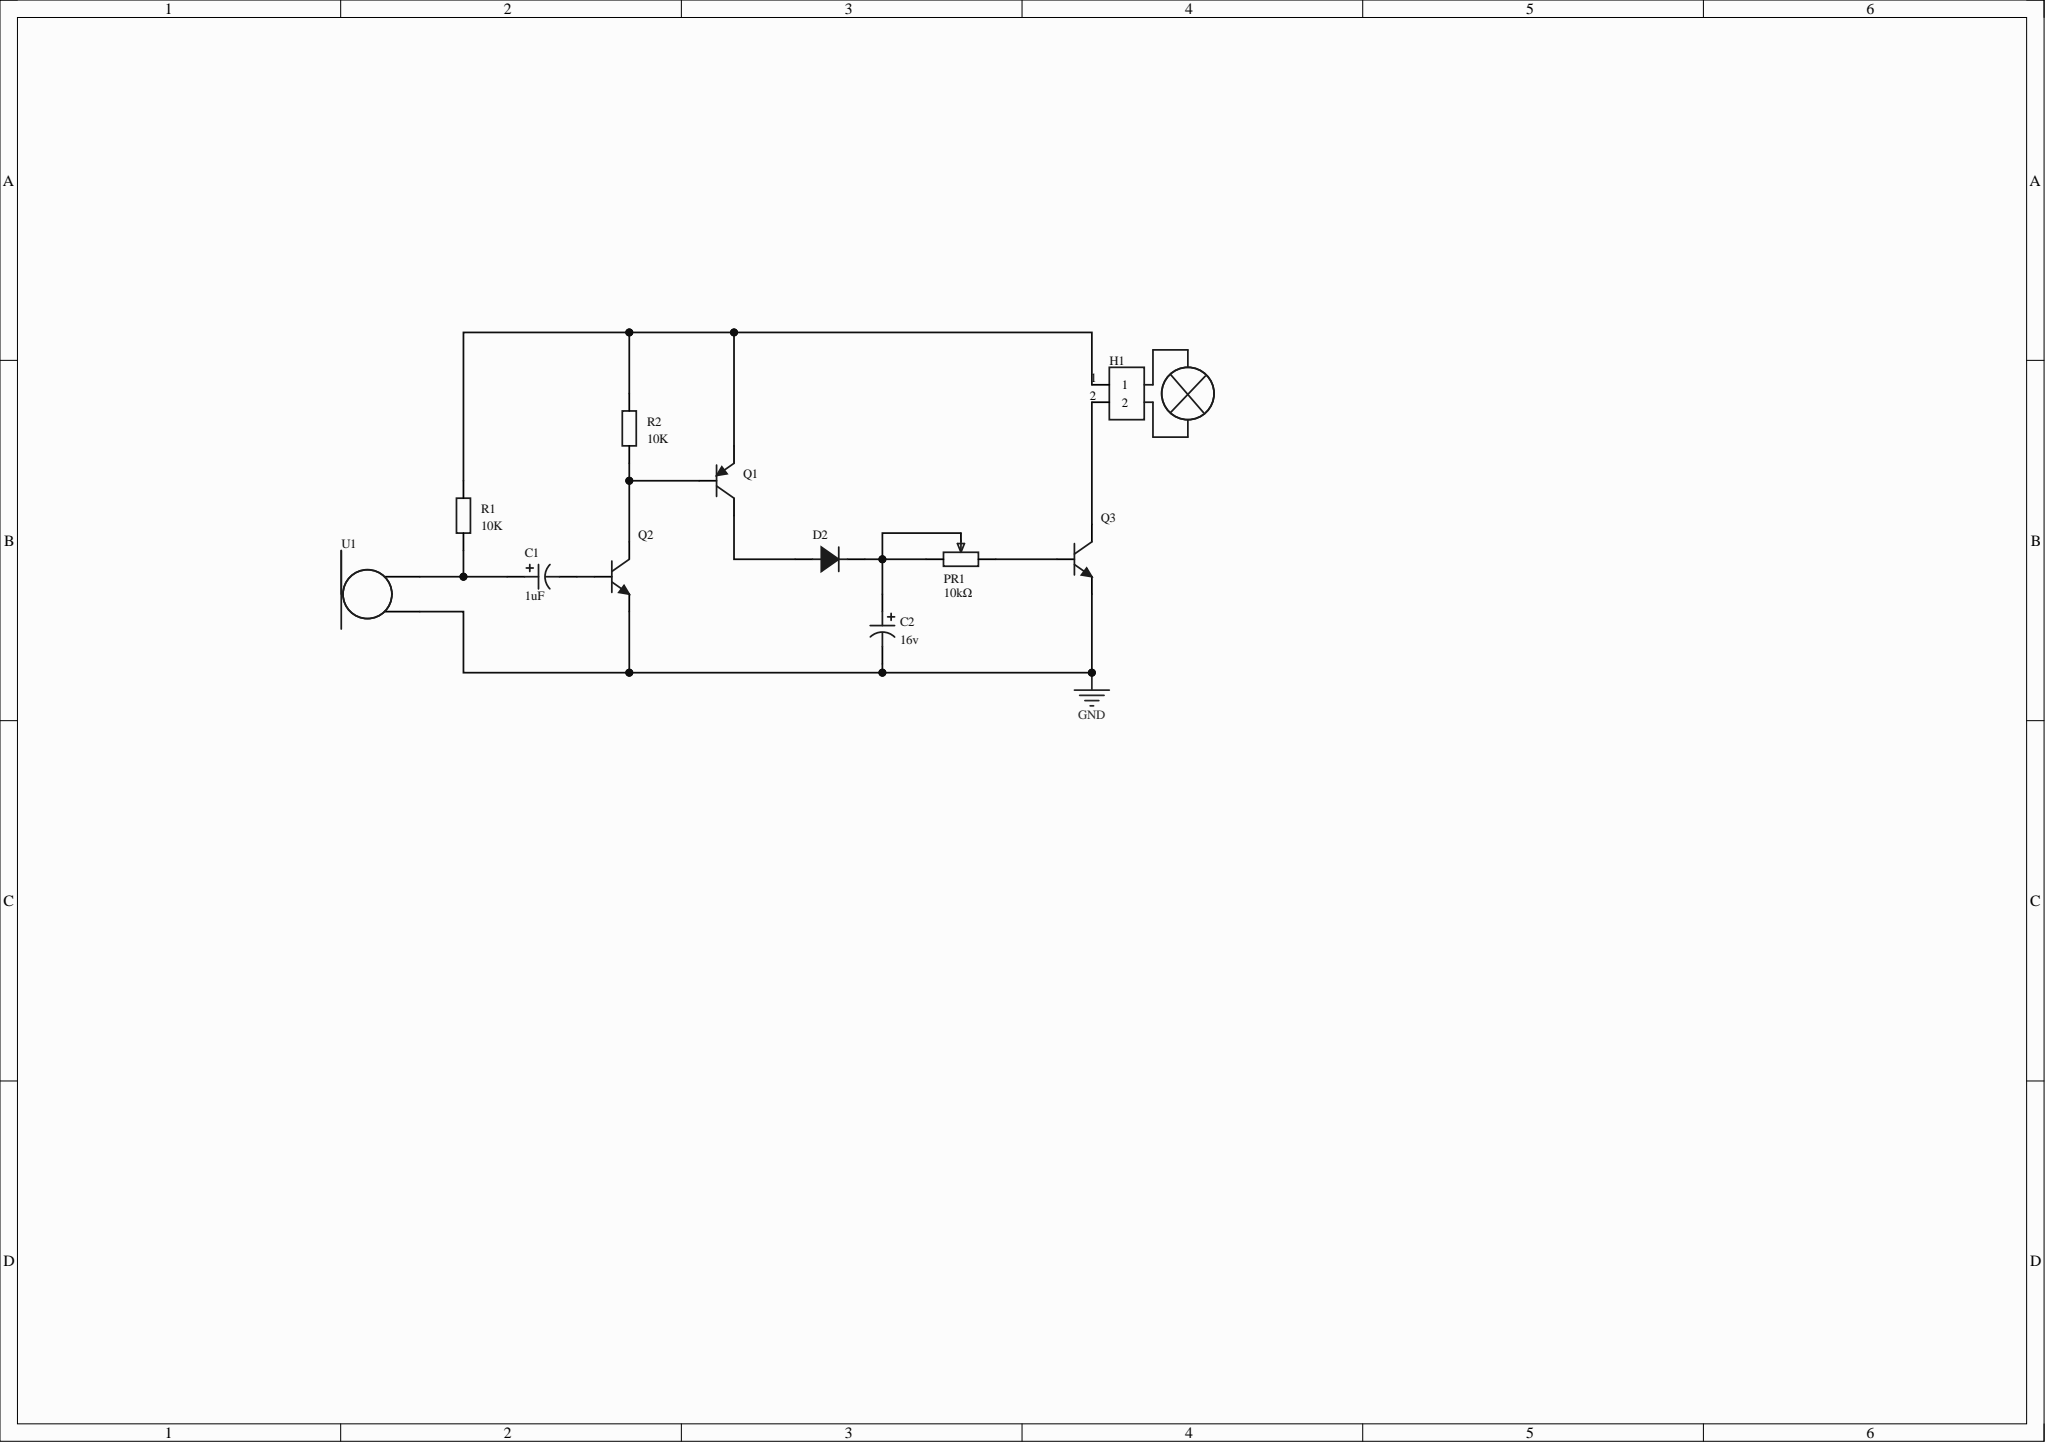Circuit board | Altium Designer | 11 parts | 9 nets
Bill of materials:
Comment,Description,Designator,Footprint,LibRef,Quantity
"1uF","Capacitance:10uF;Tolerance:±20%;Rated voltage:50V;Ripple current:120mA@100KHz;Equivalent series resistance(ESR):1.6Ω;","C1","CAP-TH_BD5.0-P2.00-D0.8-FD-10UF50VC110GL","10UF50VC110GL","1"
"16v","Capacitance:10uF;Tolerance:±20%;Rated voltage:50V;Ripple current:120mA@100KHz;Equivalent series resistance(ESR):1.6Ω;","C2","CAP-TH_BD5.0-P2.00-D0.8-FD-10UF50VC110GL","10UF50VC110GL","1"
"","","D2","SMA_1N4007","D_1N4007","1"
"","","H1","HDR-TH_2P-P2.54-V-M-1","HDR-M_2.54_1x2P","1"
"10kΩ","","PR1","R_3296","R_3296","1"
"","","Q1","S8550P_SOT","S8550_SOT_PNP","1"
"","","Q2, Q3","S8050_SOT-23","S8050_SOT_NPN","2"
"10K","","R1, R2","R0603","Res_0603","2"
"Current source","","U1","咪头","咪头","1"
Netlist (Protel format):
[
C1
CAP-TH_BD5.0-P2.00-D0.8-FD-10UF50VC110GL
1uF



]
[
C2
CAP-TH_BD5.0-P2.00-D0.8-FD-10UF50VC110GL
16v



]
[
D2
SMA_1N4007




]
[
H1
HDR-TH_2P-P2.54-V-M-1




]
[
PR1
R_3296
10kΩ



]
[
Q1
S8550P_SOT




]
[
Q2
S8050_SOT-23




]
[
Q3
S8050_SOT-23




]
[
R1
R0603
10K



]
[
R2
R0603
10K



]
[
U1
咪头
Current source



]
(
NetQ1_1
Q1-1
Q2-3
R2-1
)
(
NetPR1_1
PR1-1
Q3-1
)
(
NetH1_2
H1-2
Q3-3
)
(
NetH1_1
H1-1
Q1-2
R1-2
R2-2
)
(
NetD2_2
D2-2
Q1-3
)
(
NetC2_1
C2-1
D2-1
PR1-2
PR1-3
)
(
NetC1_2
C1-2
Q2-1
)
(
NetC1_1
C1-1
R1-1
U1-2
)
(
GND
C2-2
Q2-2
Q3-2
U1-1
)